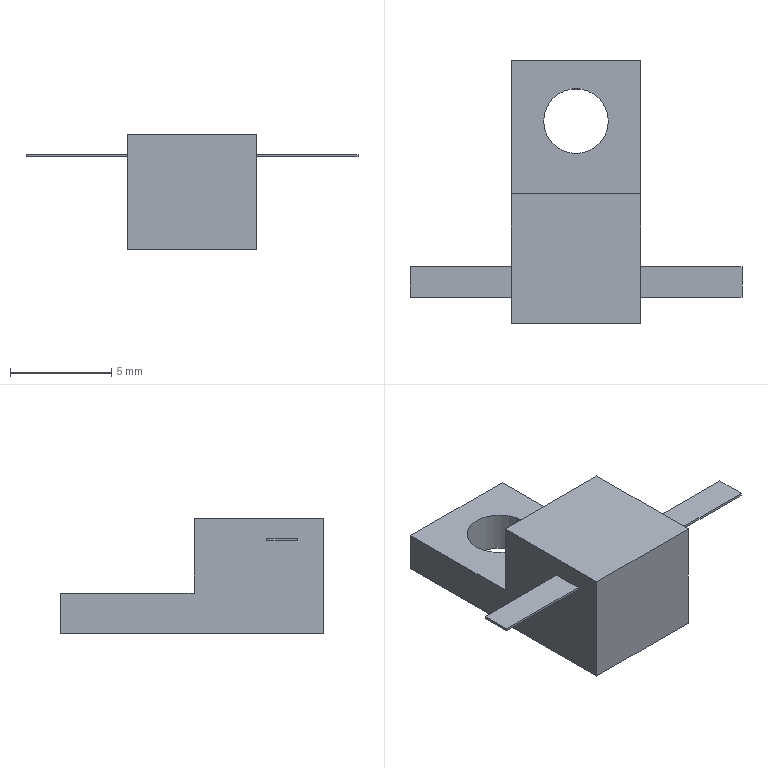Part | STEP file | RHD-50W | 1 solid | 19 faces | box 16.4 x 13 x 5.7 mm | volume 303.667 mm3 | plane 18 | cylinder 1 | commonest cylinder face diameters 3.2 x1
STEP:
#1=CARTESIAN_POINT('',(0.,0.,0.));
#2=DIRECTION('',(0.,0.,1.));
#3=DIRECTION('',(1.,0.,0.));
#4=AXIS2_PLACEMENT_3D('',#1,#2,#3);
#5=CARTESIAN_POINT('',(-120.874,-67.744,52.444));
#6=VERTEX_POINT('',#5);
#7=CARTESIAN_POINT('',(-120.874,-80.744,52.444));
#8=VERTEX_POINT('',#7);
#9=CARTESIAN_POINT('',(-120.874,-67.744,52.444));
#10=DIRECTION('',(0.,-1.,0.));
#11=VECTOR('',#10,1.);
#12=LINE('',#9,#11);
#13=CARTESIAN_POINT('',(-120.874,-67.744,54.444));
#14=DIRECTION('',(1.,0.,0.));
#15=DIRECTION('',(0.,0.,-1.));
#16=AXIS2_PLACEMENT_3D('',#13,#14,#15);
#17=PLANE('',#16);
#18=CARTESIAN_POINT('',(2.,0.));
#19=DIRECTION('',(0.,-1.));
#20=VECTOR('',#19,1.);
#21=LINE('',#18,#20);
#22=(GEOMETRIC_REPRESENTATION_CONTEXT(2)PARAMETRIC_REPRESENTATION_CONTEXT()REPRESENTATION_CONTEXT('',''));
#23=DEFINITIONAL_REPRESENTATION('',(#21),#22);
#24=PCURVE('',#17,#23);
#25=CARTESIAN_POINT('',(-117.674,-70.744,52.444));
#26=DIRECTION('',(0.,0.,1.));
#27=DIRECTION('',(1.,0.,0.));
#28=AXIS2_PLACEMENT_3D('',#25,#26,#27);
#29=PLANE('',#28);
#30=CARTESIAN_POINT('',(-3.2,3.));
#31=DIRECTION('',(0.,-1.));
#32=VECTOR('',#31,1.);
#33=LINE('',#30,#32);
#34=(GEOMETRIC_REPRESENTATION_CONTEXT(2)PARAMETRIC_REPRESENTATION_CONTEXT()REPRESENTATION_CONTEXT('',''));
#35=DEFINITIONAL_REPRESENTATION('',(#33),#34);
#36=PCURVE('',#29,#35);
#37=SURFACE_CURVE('',#12,(#24,#36),.PCURVE_S1.);
#38=EDGE_CURVE('',#6,#8,#37,.T.);
#39=ORIENTED_EDGE('',*,*,#38,.T.);
#40=CARTESIAN_POINT('',(-120.874,-80.744,58.144));
#41=VERTEX_POINT('',#40);
#42=CARTESIAN_POINT('',(-120.874,-80.744,54.444));
#43=DIRECTION('',(0.,0.,-1.));
#44=VECTOR('',#43,1.);
#45=LINE('',#42,#44);
#46=CARTESIAN_POINT('',(0.,-13.));
#47=DIRECTION('',(1.,0.));
#48=VECTOR('',#47,1.);
#49=LINE('',#46,#48);
#50=(GEOMETRIC_REPRESENTATION_CONTEXT(2)PARAMETRIC_REPRESENTATION_CONTEXT()REPRESENTATION_CONTEXT('',''));
#51=DEFINITIONAL_REPRESENTATION('',(#49),#50);
#52=PCURVE('',#17,#51);
#53=CARTESIAN_POINT('',(-120.874,-80.744,54.444));
#54=DIRECTION('',(0.,1.,0.));
#55=DIRECTION('',(0.,0.,1.));
#56=AXIS2_PLACEMENT_3D('',#53,#54,#55);
#57=PLANE('',#56);
#58=CARTESIAN_POINT('',(0.,0.));
#59=DIRECTION('',(-1.,0.));
#60=VECTOR('',#59,1.);
#61=LINE('',#58,#60);
#62=(GEOMETRIC_REPRESENTATION_CONTEXT(2)PARAMETRIC_REPRESENTATION_CONTEXT()REPRESENTATION_CONTEXT('',''));
#63=DEFINITIONAL_REPRESENTATION('',(#61),#62);
#64=PCURVE('',#57,#63);
#65=SURFACE_CURVE('',#45,(#52,#64),.PCURVE_S1.);
#66=EDGE_CURVE('',#41,#8,#65,.T.);
#67=ORIENTED_EDGE('',*,*,#66,.F.);
#68=CARTESIAN_POINT('',(-120.874,-74.344,58.144));
#69=VERTEX_POINT('',#68);
#70=CARTESIAN_POINT('',(-120.874,-74.344,58.144));
#71=DIRECTION('',(0.,-1.,0.));
#72=VECTOR('',#71,1.);
#73=LINE('',#70,#72);
#74=CARTESIAN_POINT('',(-3.7,-6.6));
#75=DIRECTION('',(0.,-1.));
#76=VECTOR('',#75,1.);
#77=LINE('',#74,#76);
#78=(GEOMETRIC_REPRESENTATION_CONTEXT(2)PARAMETRIC_REPRESENTATION_CONTEXT()REPRESENTATION_CONTEXT('',''));
#79=DEFINITIONAL_REPRESENTATION('',(#77),#78);
#80=PCURVE('',#17,#79);
#81=CARTESIAN_POINT('',(0.,0.,58.144));
#82=DIRECTION('',(0.,0.,1.));
#83=DIRECTION('',(1.,0.,0.));
#84=AXIS2_PLACEMENT_3D('',#81,#82,#83);
#85=PLANE('',#84);
#86=CARTESIAN_POINT('',(-120.874,-74.344));
#87=DIRECTION('',(0.,-1.));
#88=VECTOR('',#87,1.);
#89=LINE('',#86,#88);
#90=(GEOMETRIC_REPRESENTATION_CONTEXT(2)PARAMETRIC_REPRESENTATION_CONTEXT()REPRESENTATION_CONTEXT('',''));
#91=DEFINITIONAL_REPRESENTATION('',(#89),#90);
#92=PCURVE('',#85,#91);
#93=SURFACE_CURVE('',#73,(#80,#92),.PCURVE_S1.);
#94=EDGE_CURVE('',#69,#41,#93,.T.);
#95=ORIENTED_EDGE('',*,*,#94,.F.);
#96=CARTESIAN_POINT('',(-120.874,-74.344,54.444));
#97=VERTEX_POINT('',#96);
#98=CARTESIAN_POINT('',(-120.874,-74.344,58.144));
#99=DIRECTION('',(0.,0.,-1.));
#100=VECTOR('',#99,1.);
#101=LINE('',#98,#100);
#102=CARTESIAN_POINT('',(-3.7,-6.6));
#103=DIRECTION('',(1.,0.));
#104=VECTOR('',#103,1.);
#105=LINE('',#102,#104);
#106=(GEOMETRIC_REPRESENTATION_CONTEXT(2)PARAMETRIC_REPRESENTATION_CONTEXT()REPRESENTATION_CONTEXT('',''));
#107=DEFINITIONAL_REPRESENTATION('',(#105),#106);
#108=PCURVE('',#17,#107);
#109=CARTESIAN_POINT('',(-114.474,-74.344,58.144));
#110=DIRECTION('',(0.,-1.,0.));
#111=DIRECTION('',(0.,0.,-1.));
#112=AXIS2_PLACEMENT_3D('',#109,#110,#111);
#113=PLANE('',#112);
#114=CARTESIAN_POINT('',(0.,-6.4));
#115=DIRECTION('',(1.,0.));
#116=VECTOR('',#115,1.);
#117=LINE('',#114,#116);
#118=(GEOMETRIC_REPRESENTATION_CONTEXT(2)PARAMETRIC_REPRESENTATION_CONTEXT()REPRESENTATION_CONTEXT('',''));
#119=DEFINITIONAL_REPRESENTATION('',(#117),#118);
#120=PCURVE('',#113,#119);
#121=SURFACE_CURVE('',#101,(#108,#120),.PCURVE_S1.);
#122=EDGE_CURVE('',#69,#97,#121,.T.);
#123=ORIENTED_EDGE('',*,*,#122,.T.);
#124=CARTESIAN_POINT('',(-120.874,-67.744,54.444));
#125=VERTEX_POINT('',#124);
#126=CARTESIAN_POINT('',(-120.874,-67.744,54.444));
#127=DIRECTION('',(0.,-1.,0.));
#128=VECTOR('',#127,1.);
#129=LINE('',#126,#128);
#130=CARTESIAN_POINT('',(0.,0.));
#131=DIRECTION('',(0.,-1.));
#132=VECTOR('',#131,1.);
#133=LINE('',#130,#132);
#134=(GEOMETRIC_REPRESENTATION_CONTEXT(2)PARAMETRIC_REPRESENTATION_CONTEXT()REPRESENTATION_CONTEXT('',''));
#135=DEFINITIONAL_REPRESENTATION('',(#133),#134);
#136=PCURVE('',#17,#135);
#137=CARTESIAN_POINT('',(-117.674,-70.744,54.444));
#138=DIRECTION('',(0.,0.,1.));
#139=DIRECTION('',(1.,0.,0.));
#140=AXIS2_PLACEMENT_3D('',#137,#138,#139);
#141=PLANE('',#140);
#142=CARTESIAN_POINT('',(-3.2,3.));
#143=DIRECTION('',(0.,-1.));
#144=VECTOR('',#143,1.);
#145=LINE('',#142,#144);
#146=(GEOMETRIC_REPRESENTATION_CONTEXT(2)PARAMETRIC_REPRESENTATION_CONTEXT()REPRESENTATION_CONTEXT('',''));
#147=DEFINITIONAL_REPRESENTATION('',(#145),#146);
#148=PCURVE('',#141,#147);
#149=SURFACE_CURVE('',#129,(#136,#148),.PCURVE_S1.);
#150=EDGE_CURVE('',#125,#97,#149,.T.);
#151=ORIENTED_EDGE('',*,*,#150,.F.);
#152=CARTESIAN_POINT('',(-120.874,-67.744,54.444));
#153=DIRECTION('',(0.,0.,-1.));
#154=VECTOR('',#153,1.);
#155=LINE('',#152,#154);
#156=CARTESIAN_POINT('',(0.,0.));
#157=DIRECTION('',(1.,0.));
#158=VECTOR('',#157,1.);
#159=LINE('',#156,#158);
#160=(GEOMETRIC_REPRESENTATION_CONTEXT(2)PARAMETRIC_REPRESENTATION_CONTEXT()REPRESENTATION_CONTEXT('',''));
#161=DEFINITIONAL_REPRESENTATION('',(#159),#160);
#162=PCURVE('',#17,#161);
#163=CARTESIAN_POINT('',(-114.474,-67.744,54.444));
#164=DIRECTION('',(0.,-1.,0.));
#165=DIRECTION('',(0.,0.,-1.));
#166=AXIS2_PLACEMENT_3D('',#163,#164,#165);
#167=PLANE('',#166);
#168=CARTESIAN_POINT('',(0.,-6.4));
#169=DIRECTION('',(1.,0.));
#170=VECTOR('',#169,1.);
#171=LINE('',#168,#170);
#172=(GEOMETRIC_REPRESENTATION_CONTEXT(2)PARAMETRIC_REPRESENTATION_CONTEXT()REPRESENTATION_CONTEXT('',''));
#173=DEFINITIONAL_REPRESENTATION('',(#171),#172);
#174=PCURVE('',#167,#173);
#175=SURFACE_CURVE('',#155,(#162,#174),.PCURVE_S1.);
#176=EDGE_CURVE('',#125,#6,#175,.T.);
#177=ORIENTED_EDGE('',*,*,#176,.T.);
#178=EDGE_LOOP('',(#39,#67,#95,#123,#151,#177));
#179=FACE_BOUND('',#178,.T.);
#180=CARTESIAN_POINT('',(-120.874,-79.444,57.024));
#181=VERTEX_POINT('',#180);
#182=CARTESIAN_POINT('',(-120.874,-79.444,57.144));
#183=VERTEX_POINT('',#182);
#184=CARTESIAN_POINT('',(-120.874,-79.444,57.024));
#185=DIRECTION('',(0.,0.,1.));
#186=VECTOR('',#185,1.);
#187=LINE('',#184,#186);
#188=CARTESIAN_POINT('',(-2.58,-11.7));
#189=DIRECTION('',(-1.,0.));
#190=VECTOR('',#189,1.);
#191=LINE('',#188,#190);
#192=(GEOMETRIC_REPRESENTATION_CONTEXT(2)PARAMETRIC_REPRESENTATION_CONTEXT()REPRESENTATION_CONTEXT('',''));
#193=DEFINITIONAL_REPRESENTATION('',(#191),#192);
#194=PCURVE('',#17,#193);
#195=CARTESIAN_POINT('',(-125.874,-79.444,57.024));
#196=DIRECTION('',(0.,1.,0.));
#197=DIRECTION('',(0.,0.,1.));
#198=AXIS2_PLACEMENT_3D('',#195,#196,#197);
#199=PLANE('',#198);
#200=CARTESIAN_POINT('',(0.,5.));
#201=DIRECTION('',(1.,0.));
#202=VECTOR('',#201,1.);
#203=LINE('',#200,#202);
#204=(GEOMETRIC_REPRESENTATION_CONTEXT(2)PARAMETRIC_REPRESENTATION_CONTEXT()REPRESENTATION_CONTEXT('',''));
#205=DEFINITIONAL_REPRESENTATION('',(#203),#204);
#206=PCURVE('',#199,#205);
#207=SURFACE_CURVE('',#187,(#194,#206),.PCURVE_S1.);
#208=EDGE_CURVE('',#181,#183,#207,.T.);
#209=ORIENTED_EDGE('',*,*,#208,.F.);
#210=CARTESIAN_POINT('',(-120.874,-77.944,57.024));
#211=VERTEX_POINT('',#210);
#212=CARTESIAN_POINT('',(-120.874,-77.944,57.024));
#213=DIRECTION('',(0.,-1.,0.));
#214=VECTOR('',#213,1.);
#215=LINE('',#212,#214);
#216=CARTESIAN_POINT('',(-2.58,-10.2));
#217=DIRECTION('',(0.,-1.));
#218=VECTOR('',#217,1.);
#219=LINE('',#216,#218);
#220=(GEOMETRIC_REPRESENTATION_CONTEXT(2)PARAMETRIC_REPRESENTATION_CONTEXT()REPRESENTATION_CONTEXT('',''));
#221=DEFINITIONAL_REPRESENTATION('',(#219),#220);
#222=PCURVE('',#17,#221);
#223=CARTESIAN_POINT('',(-125.874,-77.944,57.024));
#224=DIRECTION('',(0.,0.,1.));
#225=DIRECTION('',(1.,0.,0.));
#226=AXIS2_PLACEMENT_3D('',#223,#224,#225);
#227=PLANE('',#226);
#228=CARTESIAN_POINT('',(5.,0.));
#229=DIRECTION('',(0.,-1.));
#230=VECTOR('',#229,1.);
#231=LINE('',#228,#230);
#232=(GEOMETRIC_REPRESENTATION_CONTEXT(2)PARAMETRIC_REPRESENTATION_CONTEXT()REPRESENTATION_CONTEXT('',''));
#233=DEFINITIONAL_REPRESENTATION('',(#231),#232);
#234=PCURVE('',#227,#233);
#235=SURFACE_CURVE('',#215,(#222,#234),.PCURVE_S1.);
#236=EDGE_CURVE('',#211,#181,#235,.T.);
#237=ORIENTED_EDGE('',*,*,#236,.F.);
#238=CARTESIAN_POINT('',(-120.874,-77.944,57.144));
#239=VERTEX_POINT('',#238);
#240=CARTESIAN_POINT('',(-120.874,-77.944,57.144));
#241=DIRECTION('',(0.,0.,-1.));
#242=VECTOR('',#241,1.);
#243=LINE('',#240,#242);
#244=CARTESIAN_POINT('',(-2.7,-10.2));
#245=DIRECTION('',(1.,0.));
#246=VECTOR('',#245,1.);
#247=LINE('',#244,#246);
#248=(GEOMETRIC_REPRESENTATION_CONTEXT(2)PARAMETRIC_REPRESENTATION_CONTEXT()REPRESENTATION_CONTEXT('',''));
#249=DEFINITIONAL_REPRESENTATION('',(#247),#248);
#250=PCURVE('',#17,#249);
#251=CARTESIAN_POINT('',(-125.874,-77.944,57.144));
#252=DIRECTION('',(0.,-1.,0.));
#253=DIRECTION('',(0.,0.,-1.));
#254=AXIS2_PLACEMENT_3D('',#251,#252,#253);
#255=PLANE('',#254);
#256=CARTESIAN_POINT('',(0.,5.));
#257=DIRECTION('',(1.,0.));
#258=VECTOR('',#257,1.);
#259=LINE('',#256,#258);
#260=(GEOMETRIC_REPRESENTATION_CONTEXT(2)PARAMETRIC_REPRESENTATION_CONTEXT()REPRESENTATION_CONTEXT('',''));
#261=DEFINITIONAL_REPRESENTATION('',(#259),#260);
#262=PCURVE('',#255,#261);
#263=SURFACE_CURVE('',#243,(#250,#262),.PCURVE_S1.);
#264=EDGE_CURVE('',#239,#211,#263,.T.);
#265=ORIENTED_EDGE('',*,*,#264,.F.);
#266=CARTESIAN_POINT('',(-120.874,-79.444,57.144));
#267=DIRECTION('',(0.,1.,0.));
#268=VECTOR('',#267,1.);
#269=LINE('',#266,#268);
#270=CARTESIAN_POINT('',(-2.7,-11.7));
#271=DIRECTION('',(0.,1.));
#272=VECTOR('',#271,1.);
#273=LINE('',#270,#272);
#274=(GEOMETRIC_REPRESENTATION_CONTEXT(2)PARAMETRIC_REPRESENTATION_CONTEXT()REPRESENTATION_CONTEXT('',''));
#275=DEFINITIONAL_REPRESENTATION('',(#273),#274);
#276=PCURVE('',#17,#275);
#277=CARTESIAN_POINT('',(-125.874,-79.444,57.144));
#278=DIRECTION('',(0.,0.,-1.));
#279=DIRECTION('',(-1.,0.,0.));
#280=AXIS2_PLACEMENT_3D('',#277,#278,#279);
#281=PLANE('',#280);
#282=CARTESIAN_POINT('',(-5.,0.));
#283=DIRECTION('',(0.,1.));
#284=VECTOR('',#283,1.);
#285=LINE('',#282,#284);
#286=(GEOMETRIC_REPRESENTATION_CONTEXT(2)PARAMETRIC_REPRESENTATION_CONTEXT()REPRESENTATION_CONTEXT('',''));
#287=DEFINITIONAL_REPRESENTATION('',(#285),#286);
#288=PCURVE('',#281,#287);
#289=SURFACE_CURVE('',#269,(#276,#288),.PCURVE_S1.);
#290=EDGE_CURVE('',#183,#239,#289,.T.);
#291=ORIENTED_EDGE('',*,*,#290,.F.);
#292=EDGE_LOOP('',(#209,#237,#265,#291));
#293=FACE_BOUND('',#292,.T.);
#294=ADVANCED_FACE('',(#179,#293),#17,.F.);
#295=CARTESIAN_POINT('',(-114.474,-80.744,52.444));
#296=VERTEX_POINT('',#295);
#297=CARTESIAN_POINT('',(-114.474,-67.744,52.444));
#298=VERTEX_POINT('',#297);
#299=CARTESIAN_POINT('',(-114.474,-80.744,52.444));
#300=DIRECTION('',(0.,1.,0.));
#301=VECTOR('',#300,1.);
#302=LINE('',#299,#301);
#303=CARTESIAN_POINT('',(-114.474,-80.744,54.444));
#304=DIRECTION('',(-1.,0.,0.));
#305=DIRECTION('',(0.,0.,1.));
#306=AXIS2_PLACEMENT_3D('',#303,#304,#305);
#307=PLANE('',#306);
#308=CARTESIAN_POINT('',(-2.,0.));
#309=DIRECTION('',(0.,1.));
#310=VECTOR('',#309,1.);
#311=LINE('',#308,#310);
#312=(GEOMETRIC_REPRESENTATION_CONTEXT(2)PARAMETRIC_REPRESENTATION_CONTEXT()REPRESENTATION_CONTEXT('',''));
#313=DEFINITIONAL_REPRESENTATION('',(#311),#312);
#314=PCURVE('',#307,#313);
#315=CARTESIAN_POINT('',(3.2,-10.));
#316=DIRECTION('',(0.,1.));
#317=VECTOR('',#316,1.);
#318=LINE('',#315,#317);
#319=(GEOMETRIC_REPRESENTATION_CONTEXT(2)PARAMETRIC_REPRESENTATION_CONTEXT()REPRESENTATION_CONTEXT('',''));
#320=DEFINITIONAL_REPRESENTATION('',(#318),#319);
#321=PCURVE('',#29,#320);
#322=SURFACE_CURVE('',#302,(#314,#321),.PCURVE_S1.);
#323=EDGE_CURVE('',#296,#298,#322,.T.);
#324=ORIENTED_EDGE('',*,*,#323,.T.);
#325=CARTESIAN_POINT('',(-114.474,-67.744,54.444));
#326=VERTEX_POINT('',#325);
#327=CARTESIAN_POINT('',(-114.474,-67.744,54.444));
#328=DIRECTION('',(0.,0.,-1.));
#329=VECTOR('',#328,1.);
#330=LINE('',#327,#329);
#331=CARTESIAN_POINT('',(0.,13.));
#332=DIRECTION('',(-1.,0.));
#333=VECTOR('',#332,1.);
#334=LINE('',#331,#333);
#335=(GEOMETRIC_REPRESENTATION_CONTEXT(2)PARAMETRIC_REPRESENTATION_CONTEXT()REPRESENTATION_CONTEXT('',''));
#336=DEFINITIONAL_REPRESENTATION('',(#334),#335);
#337=PCURVE('',#307,#336);
#338=CARTESIAN_POINT('',(0.,0.));
#339=DIRECTION('',(1.,0.));
#340=VECTOR('',#339,1.);
#341=LINE('',#338,#340);
#342=(GEOMETRIC_REPRESENTATION_CONTEXT(2)PARAMETRIC_REPRESENTATION_CONTEXT()REPRESENTATION_CONTEXT('',''));
#343=DEFINITIONAL_REPRESENTATION('',(#341),#342);
#344=PCURVE('',#167,#343);
#345=SURFACE_CURVE('',#330,(#337,#344),.PCURVE_S1.);
#346=EDGE_CURVE('',#326,#298,#345,.T.);
#347=ORIENTED_EDGE('',*,*,#346,.F.);
#348=CARTESIAN_POINT('',(-114.474,-74.344,54.444));
#349=VERTEX_POINT('',#348);
#350=CARTESIAN_POINT('',(-114.474,-80.744,54.444));
#351=DIRECTION('',(0.,1.,0.));
#352=VECTOR('',#351,1.);
#353=LINE('',#350,#352);
#354=CARTESIAN_POINT('',(0.,0.));
#355=DIRECTION('',(0.,1.));
#356=VECTOR('',#355,1.);
#357=LINE('',#354,#356);
#358=(GEOMETRIC_REPRESENTATION_CONTEXT(2)PARAMETRIC_REPRESENTATION_CONTEXT()REPRESENTATION_CONTEXT('',''));
#359=DEFINITIONAL_REPRESENTATION('',(#357),#358);
#360=PCURVE('',#307,#359);
#361=CARTESIAN_POINT('',(3.2,-10.));
#362=DIRECTION('',(0.,1.));
#363=VECTOR('',#362,1.);
#364=LINE('',#361,#363);
#365=(GEOMETRIC_REPRESENTATION_CONTEXT(2)PARAMETRIC_REPRESENTATION_CONTEXT()REPRESENTATION_CONTEXT('',''));
#366=DEFINITIONAL_REPRESENTATION('',(#364),#365);
#367=PCURVE('',#141,#366);
#368=SURFACE_CURVE('',#353,(#360,#367),.PCURVE_S1.);
#369=EDGE_CURVE('',#349,#326,#368,.T.);
#370=ORIENTED_EDGE('',*,*,#369,.F.);
#371=CARTESIAN_POINT('',(-114.474,-74.344,58.144));
#372=VERTEX_POINT('',#371);
#373=CARTESIAN_POINT('',(-114.474,-74.344,58.144));
#374=DIRECTION('',(0.,0.,-1.));
#375=VECTOR('',#374,1.);
#376=LINE('',#373,#375);
#377=CARTESIAN_POINT('',(3.7,6.4));
#378=DIRECTION('',(-1.,0.));
#379=VECTOR('',#378,1.);
#380=LINE('',#377,#379);
#381=(GEOMETRIC_REPRESENTATION_CONTEXT(2)PARAMETRIC_REPRESENTATION_CONTEXT()REPRESENTATION_CONTEXT('',''));
#382=DEFINITIONAL_REPRESENTATION('',(#380),#381);
#383=PCURVE('',#307,#382);
#384=CARTESIAN_POINT('',(0.,0.));
#385=DIRECTION('',(1.,0.));
#386=VECTOR('',#385,1.);
#387=LINE('',#384,#386);
#388=(GEOMETRIC_REPRESENTATION_CONTEXT(2)PARAMETRIC_REPRESENTATION_CONTEXT()REPRESENTATION_CONTEXT('',''));
#389=DEFINITIONAL_REPRESENTATION('',(#387),#388);
#390=PCURVE('',#113,#389);
#391=SURFACE_CURVE('',#376,(#383,#390),.PCURVE_S1.);
#392=EDGE_CURVE('',#372,#349,#391,.T.);
#393=ORIENTED_EDGE('',*,*,#392,.F.);
#394=CARTESIAN_POINT('',(-114.474,-80.744,58.144));
#395=VERTEX_POINT('',#394);
#396=CARTESIAN_POINT('',(-114.474,-80.744,58.144));
#397=DIRECTION('',(0.,1.,0.));
#398=VECTOR('',#397,1.);
#399=LINE('',#396,#398);
#400=CARTESIAN_POINT('',(3.7,0.));
#401=DIRECTION('',(0.,1.));
#402=VECTOR('',#401,1.);
#403=LINE('',#400,#402);
#404=(GEOMETRIC_REPRESENTATION_CONTEXT(2)PARAMETRIC_REPRESENTATION_CONTEXT()REPRESENTATION_CONTEXT('',''));
#405=DEFINITIONAL_REPRESENTATION('',(#403),#404);
#406=PCURVE('',#307,#405);
#407=CARTESIAN_POINT('',(-114.474,-80.744));
#408=DIRECTION('',(0.,1.));
#409=VECTOR('',#408,1.);
#410=LINE('',#407,#409);
#411=(GEOMETRIC_REPRESENTATION_CONTEXT(2)PARAMETRIC_REPRESENTATION_CONTEXT()REPRESENTATION_CONTEXT('',''));
#412=DEFINITIONAL_REPRESENTATION('',(#410),#411);
#413=PCURVE('',#85,#412);
#414=SURFACE_CURVE('',#399,(#406,#413),.PCURVE_S1.);
#415=EDGE_CURVE('',#395,#372,#414,.T.);
#416=ORIENTED_EDGE('',*,*,#415,.F.);
#417=CARTESIAN_POINT('',(-114.474,-80.744,54.444));
#418=DIRECTION('',(0.,0.,-1.));
#419=VECTOR('',#418,1.);
#420=LINE('',#417,#419);
#421=CARTESIAN_POINT('',(0.,0.));
#422=DIRECTION('',(-1.,0.));
#423=VECTOR('',#422,1.);
#424=LINE('',#421,#423);
#425=(GEOMETRIC_REPRESENTATION_CONTEXT(2)PARAMETRIC_REPRESENTATION_CONTEXT()REPRESENTATION_CONTEXT('',''));
#426=DEFINITIONAL_REPRESENTATION('',(#424),#425);
#427=PCURVE('',#307,#426);
#428=CARTESIAN_POINT('',(0.,6.4));
#429=DIRECTION('',(-1.,0.));
#430=VECTOR('',#429,1.);
#431=LINE('',#428,#430);
#432=(GEOMETRIC_REPRESENTATION_CONTEXT(2)PARAMETRIC_REPRESENTATION_CONTEXT()REPRESENTATION_CONTEXT('',''));
#433=DEFINITIONAL_REPRESENTATION('',(#431),#432);
#434=PCURVE('',#57,#433);
#435=SURFACE_CURVE('',#420,(#427,#434),.PCURVE_S1.);
#436=EDGE_CURVE('',#395,#296,#435,.T.);
#437=ORIENTED_EDGE('',*,*,#436,.T.);
#438=EDGE_LOOP('',(#324,#347,#370,#393,#416,#437));
#439=FACE_BOUND('',#438,.T.);
#440=CARTESIAN_POINT('',(-114.474,-79.444,57.144));
#441=VERTEX_POINT('',#440);
#442=CARTESIAN_POINT('',(-114.474,-79.444,57.024));
#443=VERTEX_POINT('',#442);
#444=CARTESIAN_POINT('',(-114.474,-79.444,57.144));
#445=DIRECTION('',(0.,0.,-1.));
#446=VECTOR('',#445,1.);
#447=LINE('',#444,#446);
#448=CARTESIAN_POINT('',(2.7,1.3));
#449=DIRECTION('',(-1.,0.));
#450=VECTOR('',#449,1.);
#451=LINE('',#448,#450);
#452=(GEOMETRIC_REPRESENTATION_CONTEXT(2)PARAMETRIC_REPRESENTATION_CONTEXT()REPRESENTATION_CONTEXT('',''));
#453=DEFINITIONAL_REPRESENTATION('',(#451),#452);
#454=PCURVE('',#307,#453);
#455=CARTESIAN_POINT('',(-109.474,-79.444,57.144));
#456=DIRECTION('',(0.,1.,0.));
#457=DIRECTION('',(0.,0.,1.));
#458=AXIS2_PLACEMENT_3D('',#455,#456,#457);
#459=PLANE('',#458);
#460=CARTESIAN_POINT('',(0.,-5.));
#461=DIRECTION('',(-1.,0.));
#462=VECTOR('',#461,1.);
#463=LINE('',#460,#462);
#464=(GEOMETRIC_REPRESENTATION_CONTEXT(2)PARAMETRIC_REPRESENTATION_CONTEXT()REPRESENTATION_CONTEXT('',''));
#465=DEFINITIONAL_REPRESENTATION('',(#463),#464);
#466=PCURVE('',#459,#465);
#467=SURFACE_CURVE('',#447,(#454,#466),.PCURVE_S1.);
#468=EDGE_CURVE('',#441,#443,#467,.T.);
#469=ORIENTED_EDGE('',*,*,#468,.F.);
#470=CARTESIAN_POINT('',(-114.474,-77.944,57.144));
#471=VERTEX_POINT('',#470);
#472=CARTESIAN_POINT('',(-114.474,-77.944,57.144));
#473=DIRECTION('',(0.,-1.,0.));
#474=VECTOR('',#473,1.);
#475=LINE('',#472,#474);
#476=CARTESIAN_POINT('',(2.7,2.8));
#477=DIRECTION('',(0.,-1.));
#478=VECTOR('',#477,1.);
#479=LINE('',#476,#478);
#480=(GEOMETRIC_REPRESENTATION_CONTEXT(2)PARAMETRIC_REPRESENTATION_CONTEXT()REPRESENTATION_CONTEXT('',''));
#481=DEFINITIONAL_REPRESENTATION('',(#479),#480);
#482=PCURVE('',#307,#481);
#483=CARTESIAN_POINT('',(-109.474,-77.944,57.144));
#484=DIRECTION('',(0.,0.,-1.));
#485=DIRECTION('',(-1.,0.,0.));
#486=AXIS2_PLACEMENT_3D('',#483,#484,#485);
#487=PLANE('',#486);
#488=CARTESIAN_POINT('',(5.,0.));
#489=DIRECTION('',(0.,-1.));
#490=VECTOR('',#489,1.);
#491=LINE('',#488,#490);
#492=(GEOMETRIC_REPRESENTATION_CONTEXT(2)PARAMETRIC_REPRESENTATION_CONTEXT()REPRESENTATION_CONTEXT('',''));
#493=DEFINITIONAL_REPRESENTATION('',(#491),#492);
#494=PCURVE('',#487,#493);
#495=SURFACE_CURVE('',#475,(#482,#494),.PCURVE_S1.);
#496=EDGE_CURVE('',#471,#441,#495,.T.);
#497=ORIENTED_EDGE('',*,*,#496,.F.);
#498=CARTESIAN_POINT('',(-114.474,-77.944,57.024));
#499=VERTEX_POINT('',#498);
#500=CARTESIAN_POINT('',(-114.474,-77.944,57.024));
#501=DIRECTION('',(0.,0.,1.));
#502=VECTOR('',#501,1.);
#503=LINE('',#500,#502);
#504=CARTESIAN_POINT('',(2.58,2.8));
#505=DIRECTION('',(1.,0.));
#506=VECTOR('',#505,1.);
#507=LINE('',#504,#506);
#508=(GEOMETRIC_REPRESENTATION_CONTEXT(2)PARAMETRIC_REPRESENTATION_CONTEXT()REPRESENTATION_CONTEXT('',''));
#509=DEFINITIONAL_REPRESENTATION('',(#507),#508);
#510=PCURVE('',#307,#509);
#511=CARTESIAN_POINT('',(-109.474,-77.944,57.024));
#512=DIRECTION('',(0.,-1.,0.));
#513=DIRECTION('',(0.,0.,-1.));
#514=AXIS2_PLACEMENT_3D('',#511,#512,#513);
#515=PLANE('',#514);
#516=CARTESIAN_POINT('',(0.,-5.));
#517=DIRECTION('',(-1.,0.));
#518=VECTOR('',#517,1.);
#519=LINE('',#516,#518);
#520=(GEOMETRIC_REPRESENTATION_CONTEXT(2)PARAMETRIC_REPRESENTATION_CONTEXT()REPRESENTATION_CONTEXT('',''));
#521=DEFINITIONAL_REPRESENTATION('',(#519),#520);
#522=PCURVE('',#515,#521);
#523=SURFACE_CURVE('',#503,(#510,#522),.PCURVE_S1.);
#524=EDGE_CURVE('',#499,#471,#523,.T.);
#525=ORIENTED_EDGE('',*,*,#524,.F.);
#526=CARTESIAN_POINT('',(-114.474,-79.444,57.024));
#527=DIRECTION('',(0.,1.,0.));
#528=VECTOR('',#527,1.);
#529=LINE('',#526,#528);
#530=CARTESIAN_POINT('',(2.58,1.3));
#531=DIRECTION('',(0.,1.));
#532=VECTOR('',#531,1.);
#533=LINE('',#530,#532);
#534=(GEOMETRIC_REPRESENTATION_CONTEXT(2)PARAMETRIC_REPRESENTATION_CONTEXT()REPRESENTATION_CONTEXT('',''));
#535=DEFINITIONAL_REPRESENTATION('',(#533),#534);
#536=PCURVE('',#307,#535);
#537=CARTESIAN_POINT('',(-109.474,-79.444,57.024));
#538=DIRECTION('',(0.,0.,1.));
#539=DIRECTION('',(1.,0.,0.));
#540=AXIS2_PLACEMENT_3D('',#537,#538,#539);
#541=PLANE('',#540);
#542=CARTESIAN_POINT('',(-5.,0.));
#543=DIRECTION('',(0.,1.));
#544=VECTOR('',#543,1.);
#545=LINE('',#542,#544);
#546=(GEOMETRIC_REPRESENTATION_CONTEXT(2)PARAMETRIC_REPRESENTATION_CONTEXT()REPRESENTATION_CONTEXT('',''));
#547=DEFINITIONAL_REPRESENTATION('',(#545),#546);
#548=PCURVE('',#541,#547);
#549=SURFACE_CURVE('',#529,(#536,#548),.PCURVE_S1.);
#550=EDGE_CURVE('',#443,#499,#549,.T.);
#551=ORIENTED_EDGE('',*,*,#550,.F.);
#552=EDGE_LOOP('',(#469,#497,#525,#551));
#553=FACE_BOUND('',#552,.T.);
#554=ADVANCED_FACE('',(#439,#553),#307,.F.);
#555=CARTESIAN_POINT('',(-120.874,-80.744,52.444));
#556=DIRECTION('',(1.,0.,0.));
#557=VECTOR('',#556,1.);
#558=LINE('',#555,#557);
#559=CARTESIAN_POINT('',(-2.,0.));
#560=DIRECTION('',(0.,1.));
#561=VECTOR('',#560,1.);
#562=LINE('',#559,#561);
#563=(GEOMETRIC_REPRESENTATION_CONTEXT(2)PARAMETRIC_REPRESENTATION_CONTEXT()REPRESENTATION_CONTEXT('',''));
#564=DEFINITIONAL_REPRESENTATION('',(#562),#563);
#565=PCURVE('',#57,#564);
#566=CARTESIAN_POINT('',(-3.2,-10.));
#567=DIRECTION('',(1.,0.));
#568=VECTOR('',#567,1.);
#569=LINE('',#566,#568);
#570=(GEOMETRIC_REPRESENTATION_CONTEXT(2)PARAMETRIC_REPRESENTATION_CONTEXT()REPRESENTATION_CONTEXT('',''));
#571=DEFINITIONAL_REPRESENTATION('',(#569),#570);
#572=PCURVE('',#29,#571);
#573=SURFACE_CURVE('',#558,(#565,#572),.PCURVE_S1.);
#574=EDGE_CURVE('',#8,#296,#573,.T.);
#575=ORIENTED_EDGE('',*,*,#574,.T.);
#576=ORIENTED_EDGE('',*,*,#436,.F.);
#577=CARTESIAN_POINT('',(-120.874,-80.744,58.144));
#578=DIRECTION('',(1.,0.,0.));
#579=VECTOR('',#578,1.);
#580=LINE('',#577,#579);
#581=CARTESIAN_POINT('',(3.7,0.));
#582=DIRECTION('',(0.,1.));
#583=VECTOR('',#582,1.);
#584=LINE('',#581,#583);
#585=(GEOMETRIC_REPRESENTATION_CONTEXT(2)PARAMETRIC_REPRESENTATION_CONTEXT()REPRESENTATION_CONTEXT('',''));
#586=DEFINITIONAL_REPRESENTATION('',(#584),#585);
#587=PCURVE('',#57,#586);
#588=CARTESIAN_POINT('',(-120.874,-80.744));
#589=DIRECTION('',(1.,0.));
#590=VECTOR('',#589,1.);
#591=LINE('',#588,#590);
#592=(GEOMETRIC_REPRESENTATION_CONTEXT(2)PARAMETRIC_REPRESENTATION_CONTEXT()REPRESENTATION_CONTEXT('',''));
#593=DEFINITIONAL_REPRESENTATION('',(#591),#592);
#594=PCURVE('',#85,#593);
#595=SURFACE_CURVE('',#580,(#587,#594),.PCURVE_S1.);
#596=EDGE_CURVE('',#41,#395,#595,.T.);
#597=ORIENTED_EDGE('',*,*,#596,.F.);
#598=ORIENTED_EDGE('',*,*,#66,.T.);
#599=EDGE_LOOP('',(#575,#576,#597,#598));
#600=FACE_BOUND('',#599,.T.);
#601=ADVANCED_FACE('',(#600),#57,.F.);
#602=CARTESIAN_POINT('',(-114.474,-67.744,52.444));
#603=DIRECTION('',(-1.,0.,0.));
#604=VECTOR('',#603,1.);
#605=LINE('',#602,#604);
#606=CARTESIAN_POINT('',(2.,0.));
#607=DIRECTION('',(0.,-1.));
#608=VECTOR('',#607,1.);
#609=LINE('',#606,#608);
#610=(GEOMETRIC_REPRESENTATION_CONTEXT(2)PARAMETRIC_REPRESENTATION_CONTEXT()REPRESENTATION_CONTEXT('',''));
#611=DEFINITIONAL_REPRESENTATION('',(#609),#610);
#612=PCURVE('',#167,#611);
#613=CARTESIAN_POINT('',(3.2,3.));
#614=DIRECTION('',(-1.,0.));
#615=VECTOR('',#614,1.);
#616=LINE('',#613,#615);
#617=(GEOMETRIC_REPRESENTATION_CONTEXT(2)PARAMETRIC_REPRESENTATION_CONTEXT()REPRESENTATION_CONTEXT('',''));
#618=DEFINITIONAL_REPRESENTATION('',(#616),#617);
#619=PCURVE('',#29,#618);
#620=SURFACE_CURVE('',#605,(#612,#619),.PCURVE_S1.);
#621=EDGE_CURVE('',#298,#6,#620,.T.);
#622=ORIENTED_EDGE('',*,*,#621,.T.);
#623=ORIENTED_EDGE('',*,*,#176,.F.);
#624=CARTESIAN_POINT('',(-114.474,-67.744,54.444));
#625=DIRECTION('',(-1.,0.,0.));
#626=VECTOR('',#625,1.);
#627=LINE('',#624,#626);
#628=CARTESIAN_POINT('',(0.,0.));
#629=DIRECTION('',(0.,-1.));
#630=VECTOR('',#629,1.);
#631=LINE('',#628,#630);
#632=(GEOMETRIC_REPRESENTATION_CONTEXT(2)PARAMETRIC_REPRESENTATION_CONTEXT()REPRESENTATION_CONTEXT('',''));
#633=DEFINITIONAL_REPRESENTATION('',(#631),#632);
#634=PCURVE('',#167,#633);
#635=CARTESIAN_POINT('',(3.2,3.));
#636=DIRECTION('',(-1.,0.));
#637=VECTOR('',#636,1.);
#638=LINE('',#635,#637);
#639=(GEOMETRIC_REPRESENTATION_CONTEXT(2)PARAMETRIC_REPRESENTATION_CONTEXT()REPRESENTATION_CONTEXT('',''));
#640=DEFINITIONAL_REPRESENTATION('',(#638),#639);
#641=PCURVE('',#141,#640);
#642=SURFACE_CURVE('',#627,(#634,#641),.PCURVE_S1.);
#643=EDGE_CURVE('',#326,#125,#642,.T.);
#644=ORIENTED_EDGE('',*,*,#643,.F.);
#645=ORIENTED_EDGE('',*,*,#346,.T.);
#646=EDGE_LOOP('',(#622,#623,#644,#645));
#647=FACE_BOUND('',#646,.T.);
#648=ADVANCED_FACE('',(#647),#167,.F.);
#649=CARTESIAN_POINT('',(-119.274,-70.744,54.444));
#650=VERTEX_POINT('',#649);
#651=CARTESIAN_POINT('',(-117.674,-70.744,54.444));
#652=DIRECTION('',(0.,0.,1.));
#653=DIRECTION('',(-1.,0.,0.));
#654=AXIS2_PLACEMENT_3D('',#651,#652,#653);
#655=CIRCLE('',#654,1.6);
#656=CARTESIAN_POINT('',(-117.674,-70.744,54.444));
#657=DIRECTION('',(0.,0.,-1.));
#658=DIRECTION('',(-1.,0.,0.));
#659=AXIS2_PLACEMENT_3D('',#656,#657,#658);
#660=CYLINDRICAL_SURFACE('',#659,1.6);
#661=CARTESIAN_POINT('',(6.283,0.));
#662=DIRECTION('',(-1.,0.));
#663=VECTOR('',#662,1.);
#664=LINE('',#661,#663);
#665=(GEOMETRIC_REPRESENTATION_CONTEXT(2)PARAMETRIC_REPRESENTATION_CONTEXT()REPRESENTATION_CONTEXT('',''));
#666=DEFINITIONAL_REPRESENTATION('',(#664),#665);
#667=PCURVE('',#660,#666);
#668=CARTESIAN_POINT('',(0.,0.));
#669=DIRECTION('',(-1.,0.));
#670=AXIS2_PLACEMENT_2D('',#668,#669);
#671=CIRCLE('',#670,1.6);
#672=(GEOMETRIC_REPRESENTATION_CONTEXT(2)PARAMETRIC_REPRESENTATION_CONTEXT()REPRESENTATION_CONTEXT('',''));
#673=DEFINITIONAL_REPRESENTATION('',(#671),#672);
#674=PCURVE('',#141,#673);
#675=SURFACE_CURVE('',#655,(#667,#674),.PCURVE_S1.);
#676=EDGE_CURVE('',#650,#650,#675,.T.);
#677=ORIENTED_EDGE('',*,*,#676,.F.);
#678=CARTESIAN_POINT('',(-119.274,-70.744,52.444));
#679=VERTEX_POINT('',#678);
#680=CARTESIAN_POINT('',(-119.274,-70.744,54.444));
#681=CARTESIAN_POINT('',(-119.274,-70.744,52.444));
#682=B_SPLINE_CURVE_WITH_KNOTS('',1,(#680,#681),.UNSPECIFIED.,.F.,.F.,(2,2),(0.,2.),.PIECEWISE_BEZIER_KNOTS.);
#683=CARTESIAN_POINT('',(6.283,0.));
#684=DIRECTION('',(0.,1.));
#685=VECTOR('',#684,1.);
#686=LINE('',#683,#685);
#687=(GEOMETRIC_REPRESENTATION_CONTEXT(2)PARAMETRIC_REPRESENTATION_CONTEXT()REPRESENTATION_CONTEXT('',''));
#688=DEFINITIONAL_REPRESENTATION('',(#686),#687);
#689=PCURVE('',#660,#688);
#690=CARTESIAN_POINT('',(0.,0.));
#691=DIRECTION('',(0.,1.));
#692=VECTOR('',#691,1.);
#693=LINE('',#690,#692);
#694=(GEOMETRIC_REPRESENTATION_CONTEXT(2)PARAMETRIC_REPRESENTATION_CONTEXT()REPRESENTATION_CONTEXT('',''));
#695=DEFINITIONAL_REPRESENTATION('',(#693),#694);
#696=PCURVE('',#660,#695);
#697=SEAM_CURVE('',#682,(#689,#696),.PCURVE_S1.);
#698=EDGE_CURVE('',#650,#679,#697,.T.);
#699=ORIENTED_EDGE('',*,*,#698,.T.);
#700=CARTESIAN_POINT('',(-117.674,-70.744,52.444));
#701=DIRECTION('',(0.,0.,1.));
#702=DIRECTION('',(-1.,0.,0.));
#703=AXIS2_PLACEMENT_3D('',#700,#701,#702);
#704=CIRCLE('',#703,1.6);
#705=CARTESIAN_POINT('',(6.283,2.));
#706=DIRECTION('',(-1.,0.));
#707=VECTOR('',#706,1.);
#708=LINE('',#705,#707);
#709=(GEOMETRIC_REPRESENTATION_CONTEXT(2)PARAMETRIC_REPRESENTATION_CONTEXT()REPRESENTATION_CONTEXT('',''));
#710=DEFINITIONAL_REPRESENTATION('',(#708),#709);
#711=PCURVE('',#660,#710);
#712=CARTESIAN_POINT('',(0.,0.));
#713=DIRECTION('',(-1.,0.));
#714=AXIS2_PLACEMENT_2D('',#712,#713);
#715=CIRCLE('',#714,1.6);
#716=(GEOMETRIC_REPRESENTATION_CONTEXT(2)PARAMETRIC_REPRESENTATION_CONTEXT()REPRESENTATION_CONTEXT('',''));
#717=DEFINITIONAL_REPRESENTATION('',(#715),#716);
#718=PCURVE('',#29,#717);
#719=SURFACE_CURVE('',#704,(#711,#718),.PCURVE_S1.);
#720=EDGE_CURVE('',#679,#679,#719,.T.);
#721=ORIENTED_EDGE('',*,*,#720,.T.);
#722=ORIENTED_EDGE('',*,*,#698,.F.);
#723=EDGE_LOOP('',(#677,#699,#721,#722));
#724=FACE_BOUND('',#723,.F.);
#725=ADVANCED_FACE('',(#724),#660,.F.);
#726=CARTESIAN_POINT('',(-114.474,-74.344,54.444));
#727=DIRECTION('',(-1.,0.,0.));
#728=VECTOR('',#727,1.);
#729=LINE('',#726,#728);
#730=CARTESIAN_POINT('',(3.2,-3.6));
#731=DIRECTION('',(-1.,0.));
#732=VECTOR('',#731,1.);
#733=LINE('',#730,#732);
#734=(GEOMETRIC_REPRESENTATION_CONTEXT(2)PARAMETRIC_REPRESENTATION_CONTEXT()REPRESENTATION_CONTEXT('',''));
#735=DEFINITIONAL_REPRESENTATION('',(#733),#734);
#736=PCURVE('',#141,#735);
#737=CARTESIAN_POINT('',(3.7,0.));
#738=DIRECTION('',(0.,-1.));
#739=VECTOR('',#738,1.);
#740=LINE('',#737,#739);
#741=(GEOMETRIC_REPRESENTATION_CONTEXT(2)PARAMETRIC_REPRESENTATION_CONTEXT()REPRESENTATION_CONTEXT('',''));
#742=DEFINITIONAL_REPRESENTATION('',(#740),#741);
#743=PCURVE('',#113,#742);
#744=SURFACE_CURVE('',#729,(#736,#743),.PCURVE_S1.);
#745=EDGE_CURVE('',#349,#97,#744,.T.);
#746=ORIENTED_EDGE('',*,*,#745,.F.);
#747=ORIENTED_EDGE('',*,*,#369,.T.);
#748=ORIENTED_EDGE('',*,*,#643,.T.);
#749=ORIENTED_EDGE('',*,*,#150,.T.);
#750=EDGE_LOOP('',(#746,#747,#748,#749));
#751=FACE_BOUND('',#750,.T.);
#752=ORIENTED_EDGE('',*,*,#676,.F.);
#753=EDGE_LOOP('',(#752));
#754=FACE_BOUND('',#753,.T.);
#755=ADVANCED_FACE('',(#751,#754),#141,.T.);
#756=ORIENTED_EDGE('',*,*,#38,.F.);
#757=ORIENTED_EDGE('',*,*,#621,.F.);
#758=ORIENTED_EDGE('',*,*,#323,.F.);
#759=ORIENTED_EDGE('',*,*,#574,.F.);
#760=EDGE_LOOP('',(#756,#757,#758,#759));
#761=FACE_BOUND('',#760,.T.);
#762=ORIENTED_EDGE('',*,*,#720,.T.);
#763=EDGE_LOOP('',(#762));
#764=FACE_BOUND('',#763,.T.);
#765=ADVANCED_FACE('',(#761,#764),#29,.F.);
#766=ORIENTED_EDGE('',*,*,#745,.T.);
#767=ORIENTED_EDGE('',*,*,#122,.F.);
#768=CARTESIAN_POINT('',(-114.474,-74.344,58.144));
#769=DIRECTION('',(-1.,0.,0.));
#770=VECTOR('',#769,1.);
#771=LINE('',#768,#770);
#772=CARTESIAN_POINT('',(0.,0.));
#773=DIRECTION('',(0.,-1.));
#774=VECTOR('',#773,1.);
#775=LINE('',#772,#774);
#776=(GEOMETRIC_REPRESENTATION_CONTEXT(2)PARAMETRIC_REPRESENTATION_CONTEXT()REPRESENTATION_CONTEXT('',''));
#777=DEFINITIONAL_REPRESENTATION('',(#775),#776);
#778=PCURVE('',#113,#777);
#779=CARTESIAN_POINT('',(-114.474,-74.344));
#780=DIRECTION('',(-1.,0.));
#781=VECTOR('',#780,1.);
#782=LINE('',#779,#781);
#783=(GEOMETRIC_REPRESENTATION_CONTEXT(2)PARAMETRIC_REPRESENTATION_CONTEXT()REPRESENTATION_CONTEXT('',''));
#784=DEFINITIONAL_REPRESENTATION('',(#782),#783);
#785=PCURVE('',#85,#784);
#786=SURFACE_CURVE('',#771,(#778,#785),.PCURVE_S1.);
#787=EDGE_CURVE('',#372,#69,#786,.T.);
#788=ORIENTED_EDGE('',*,*,#787,.F.);
#789=ORIENTED_EDGE('',*,*,#392,.T.);
#790=EDGE_LOOP('',(#766,#767,#788,#789));
#791=FACE_BOUND('',#790,.T.);
#792=ADVANCED_FACE('',(#791),#113,.F.);
#793=ORIENTED_EDGE('',*,*,#94,.T.);
#794=ORIENTED_EDGE('',*,*,#596,.T.);
#795=ORIENTED_EDGE('',*,*,#415,.T.);
#796=ORIENTED_EDGE('',*,*,#787,.T.);
#797=EDGE_LOOP('',(#793,#794,#795,#796));
#798=FACE_BOUND('',#797,.T.);
#799=ADVANCED_FACE('',(#798),#85,.T.);
#800=ORIENTED_EDGE('',*,*,#468,.T.);
#801=CARTESIAN_POINT('',(-109.474,-79.444,57.024));
#802=VERTEX_POINT('',#801);
#803=CARTESIAN_POINT('',(-109.474,-79.444,57.024));
#804=DIRECTION('',(-1.,0.,0.));
#805=VECTOR('',#804,1.);
#806=LINE('',#803,#805);
#807=CARTESIAN_POINT('',(-0.12,0.));
#808=DIRECTION('',(0.,-1.));
#809=VECTOR('',#808,1.);
#810=LINE('',#807,#809);
#811=(GEOMETRIC_REPRESENTATION_CONTEXT(2)PARAMETRIC_REPRESENTATION_CONTEXT()REPRESENTATION_CONTEXT('',''));
#812=DEFINITIONAL_REPRESENTATION('',(#810),#811);
#813=PCURVE('',#459,#812);
#814=CARTESIAN_POINT('',(0.,0.));
#815=DIRECTION('',(-1.,0.));
#816=VECTOR('',#815,1.);
#817=LINE('',#814,#816);
#818=(GEOMETRIC_REPRESENTATION_CONTEXT(2)PARAMETRIC_REPRESENTATION_CONTEXT()REPRESENTATION_CONTEXT('',''));
#819=DEFINITIONAL_REPRESENTATION('',(#817),#818);
#820=PCURVE('',#541,#819);
#821=SURFACE_CURVE('',#806,(#813,#820),.PCURVE_S1.);
#822=EDGE_CURVE('',#802,#443,#821,.T.);
#823=ORIENTED_EDGE('',*,*,#822,.F.);
#824=CARTESIAN_POINT('',(-109.474,-79.444,57.144));
#825=VERTEX_POINT('',#824);
#826=CARTESIAN_POINT('',(-109.474,-79.444,57.144));
#827=DIRECTION('',(0.,0.,-1.));
#828=VECTOR('',#827,1.);
#829=LINE('',#826,#828);
#830=CARTESIAN_POINT('',(0.,0.));
#831=DIRECTION('',(-1.,0.));
#832=VECTOR('',#831,1.);
#833=LINE('',#830,#832);
#834=(GEOMETRIC_REPRESENTATION_CONTEXT(2)PARAMETRIC_REPRESENTATION_CONTEXT()REPRESENTATION_CONTEXT('',''));
#835=DEFINITIONAL_REPRESENTATION('',(#833),#834);
#836=PCURVE('',#459,#835);
#837=CARTESIAN_POINT('',(-109.474,0.,0.));
#838=DIRECTION('',(1.,0.,0.));
#839=DIRECTION('',(0.,0.,-1.));
#840=AXIS2_PLACEMENT_3D('',#837,#838,#839);
#841=PLANE('',#840);
#842=CARTESIAN_POINT('',(-57.144,-79.444));
#843=DIRECTION('',(1.,0.));
#844=VECTOR('',#843,1.);
#845=LINE('',#842,#844);
#846=(GEOMETRIC_REPRESENTATION_CONTEXT(2)PARAMETRIC_REPRESENTATION_CONTEXT()REPRESENTATION_CONTEXT('',''));
#847=DEFINITIONAL_REPRESENTATION('',(#845),#846);
#848=PCURVE('',#841,#847);
#849=SURFACE_CURVE('',#829,(#836,#848),.PCURVE_S1.);
#850=EDGE_CURVE('',#825,#802,#849,.T.);
#851=ORIENTED_EDGE('',*,*,#850,.F.);
#852=CARTESIAN_POINT('',(-109.474,-79.444,57.144));
#853=DIRECTION('',(-1.,0.,0.));
#854=VECTOR('',#853,1.);
#855=LINE('',#852,#854);
#856=CARTESIAN_POINT('',(0.,0.));
#857=DIRECTION('',(0.,-1.));
#858=VECTOR('',#857,1.);
#859=LINE('',#856,#858);
#860=(GEOMETRIC_REPRESENTATION_CONTEXT(2)PARAMETRIC_REPRESENTATION_CONTEXT()REPRESENTATION_CONTEXT('',''));
#861=DEFINITIONAL_REPRESENTATION('',(#859),#860);
#862=PCURVE('',#459,#861);
#863=CARTESIAN_POINT('',(0.,-1.5));
#864=DIRECTION('',(1.,0.));
#865=VECTOR('',#864,1.);
#866=LINE('',#863,#865);
#867=(GEOMETRIC_REPRESENTATION_CONTEXT(2)PARAMETRIC_REPRESENTATION_CONTEXT()REPRESENTATION_CONTEXT('',''));
#868=DEFINITIONAL_REPRESENTATION('',(#866),#867);
#869=PCURVE('',#487,#868);
#870=SURFACE_CURVE('',#855,(#862,#869),.PCURVE_S1.);
#871=EDGE_CURVE('',#825,#441,#870,.T.);
#872=ORIENTED_EDGE('',*,*,#871,.T.);
#873=EDGE_LOOP('',(#800,#823,#851,#872));
#874=FACE_BOUND('',#873,.T.);
#875=ADVANCED_FACE('',(#874),#459,.F.);
#876=ORIENTED_EDGE('',*,*,#550,.T.);
#877=CARTESIAN_POINT('',(-109.474,-77.944,57.024));
#878=VERTEX_POINT('',#877);
#879=CARTESIAN_POINT('',(-109.474,-77.944,57.024));
#880=DIRECTION('',(-1.,0.,0.));
#881=VECTOR('',#880,1.);
#882=LINE('',#879,#881);
#883=CARTESIAN_POINT('',(0.,1.5));
#884=DIRECTION('',(-1.,0.));
#885=VECTOR('',#884,1.);
#886=LINE('',#883,#885);
#887=(GEOMETRIC_REPRESENTATION_CONTEXT(2)PARAMETRIC_REPRESENTATION_CONTEXT()REPRESENTATION_CONTEXT('',''));
#888=DEFINITIONAL_REPRESENTATION('',(#886),#887);
#889=PCURVE('',#541,#888);
#890=CARTESIAN_POINT('',(0.,0.));
#891=DIRECTION('',(0.,-1.));
#892=VECTOR('',#891,1.);
#893=LINE('',#890,#892);
#894=(GEOMETRIC_REPRESENTATION_CONTEXT(2)PARAMETRIC_REPRESENTATION_CONTEXT()REPRESENTATION_CONTEXT('',''));
#895=DEFINITIONAL_REPRESENTATION('',(#893),#894);
#896=PCURVE('',#515,#895);
#897=SURFACE_CURVE('',#882,(#889,#896),.PCURVE_S1.);
#898=EDGE_CURVE('',#878,#499,#897,.T.);
#899=ORIENTED_EDGE('',*,*,#898,.F.);
#900=CARTESIAN_POINT('',(-109.474,-79.444,57.024));
#901=DIRECTION('',(0.,1.,0.));
#902=VECTOR('',#901,1.);
#903=LINE('',#900,#902);
#904=CARTESIAN_POINT('',(0.,0.));
#905=DIRECTION('',(0.,1.));
#906=VECTOR('',#905,1.);
#907=LINE('',#904,#906);
#908=(GEOMETRIC_REPRESENTATION_CONTEXT(2)PARAMETRIC_REPRESENTATION_CONTEXT()REPRESENTATION_CONTEXT('',''));
#909=DEFINITIONAL_REPRESENTATION('',(#907),#908);
#910=PCURVE('',#541,#909);
#911=CARTESIAN_POINT('',(-57.024,-79.444));
#912=DIRECTION('',(0.,1.));
#913=VECTOR('',#912,1.);
#914=LINE('',#911,#913);
#915=(GEOMETRIC_REPRESENTATION_CONTEXT(2)PARAMETRIC_REPRESENTATION_CONTEXT()REPRESENTATION_CONTEXT('',''));
#916=DEFINITIONAL_REPRESENTATION('',(#914),#915);
#917=PCURVE('',#841,#916);
#918=SURFACE_CURVE('',#903,(#910,#917),.PCURVE_S1.);
#919=EDGE_CURVE('',#802,#878,#918,.T.);
#920=ORIENTED_EDGE('',*,*,#919,.F.);
#921=ORIENTED_EDGE('',*,*,#822,.T.);
#922=EDGE_LOOP('',(#876,#899,#920,#921));
#923=FACE_BOUND('',#922,.T.);
#924=ADVANCED_FACE('',(#923),#541,.F.);
#925=ORIENTED_EDGE('',*,*,#524,.T.);
#926=CARTESIAN_POINT('',(-109.474,-77.944,57.144));
#927=VERTEX_POINT('',#926);
#928=CARTESIAN_POINT('',(-109.474,-77.944,57.144));
#929=DIRECTION('',(-1.,0.,0.));
#930=VECTOR('',#929,1.);
#931=LINE('',#928,#930);
#932=CARTESIAN_POINT('',(-0.12,0.));
#933=DIRECTION('',(0.,-1.));
#934=VECTOR('',#933,1.);
#935=LINE('',#932,#934);
#936=(GEOMETRIC_REPRESENTATION_CONTEXT(2)PARAMETRIC_REPRESENTATION_CONTEXT()REPRESENTATION_CONTEXT('',''));
#937=DEFINITIONAL_REPRESENTATION('',(#935),#936);
#938=PCURVE('',#515,#937);
#939=CARTESIAN_POINT('',(0.,0.));
#940=DIRECTION('',(1.,0.));
#941=VECTOR('',#940,1.);
#942=LINE('',#939,#941);
#943=(GEOMETRIC_REPRESENTATION_CONTEXT(2)PARAMETRIC_REPRESENTATION_CONTEXT()REPRESENTATION_CONTEXT('',''));
#944=DEFINITIONAL_REPRESENTATION('',(#942),#943);
#945=PCURVE('',#487,#944);
#946=SURFACE_CURVE('',#931,(#938,#945),.PCURVE_S1.);
#947=EDGE_CURVE('',#927,#471,#946,.T.);
#948=ORIENTED_EDGE('',*,*,#947,.F.);
#949=CARTESIAN_POINT('',(-109.474,-77.944,57.024));
#950=DIRECTION('',(0.,0.,1.));
#951=VECTOR('',#950,1.);
#952=LINE('',#949,#951);
#953=CARTESIAN_POINT('',(0.,0.));
#954=DIRECTION('',(-1.,0.));
#955=VECTOR('',#954,1.);
#956=LINE('',#953,#955);
#957=(GEOMETRIC_REPRESENTATION_CONTEXT(2)PARAMETRIC_REPRESENTATION_CONTEXT()REPRESENTATION_CONTEXT('',''));
#958=DEFINITIONAL_REPRESENTATION('',(#956),#957);
#959=PCURVE('',#515,#958);
#960=CARTESIAN_POINT('',(-57.024,-77.944));
#961=DIRECTION('',(-1.,0.));
#962=VECTOR('',#961,1.);
#963=LINE('',#960,#962);
#964=(GEOMETRIC_REPRESENTATION_CONTEXT(2)PARAMETRIC_REPRESENTATION_CONTEXT()REPRESENTATION_CONTEXT('',''));
#965=DEFINITIONAL_REPRESENTATION('',(#963),#964);
#966=PCURVE('',#841,#965);
#967=SURFACE_CURVE('',#952,(#959,#966),.PCURVE_S1.);
#968=EDGE_CURVE('',#878,#927,#967,.T.);
#969=ORIENTED_EDGE('',*,*,#968,.F.);
#970=ORIENTED_EDGE('',*,*,#898,.T.);
#971=EDGE_LOOP('',(#925,#948,#969,#970));
#972=FACE_BOUND('',#971,.T.);
#973=ADVANCED_FACE('',(#972),#515,.F.);
#974=ORIENTED_EDGE('',*,*,#496,.T.);
#975=ORIENTED_EDGE('',*,*,#871,.F.);
#976=CARTESIAN_POINT('',(-109.474,-77.944,57.144));
#977=DIRECTION('',(0.,-1.,0.));
#978=VECTOR('',#977,1.);
#979=LINE('',#976,#978);
#980=CARTESIAN_POINT('',(0.,0.));
#981=DIRECTION('',(0.,-1.));
#982=VECTOR('',#981,1.);
#983=LINE('',#980,#982);
#984=(GEOMETRIC_REPRESENTATION_CONTEXT(2)PARAMETRIC_REPRESENTATION_CONTEXT()REPRESENTATION_CONTEXT('',''));
#985=DEFINITIONAL_REPRESENTATION('',(#983),#984);
#986=PCURVE('',#487,#985);
#987=CARTESIAN_POINT('',(-57.144,-77.944));
#988=DIRECTION('',(0.,-1.));
#989=VECTOR('',#988,1.);
#990=LINE('',#987,#989);
#991=(GEOMETRIC_REPRESENTATION_CONTEXT(2)PARAMETRIC_REPRESENTATION_CONTEXT()REPRESENTATION_CONTEXT('',''));
#992=DEFINITIONAL_REPRESENTATION('',(#990),#991);
#993=PCURVE('',#841,#992);
#994=SURFACE_CURVE('',#979,(#986,#993),.PCURVE_S1.);
#995=EDGE_CURVE('',#927,#825,#994,.T.);
#996=ORIENTED_EDGE('',*,*,#995,.F.);
#997=ORIENTED_EDGE('',*,*,#947,.T.);
#998=EDGE_LOOP('',(#974,#975,#996,#997));
#999=FACE_BOUND('',#998,.T.);
#1000=ADVANCED_FACE('',(#999),#487,.F.);
#1001=ORIENTED_EDGE('',*,*,#850,.T.);
#1002=ORIENTED_EDGE('',*,*,#919,.T.);
#1003=ORIENTED_EDGE('',*,*,#968,.T.);
#1004=ORIENTED_EDGE('',*,*,#995,.T.);
#1005=EDGE_LOOP('',(#1001,#1002,#1003,#1004));
#1006=FACE_BOUND('',#1005,.T.);
#1007=ADVANCED_FACE('',(#1006),#841,.T.);
#1008=ORIENTED_EDGE('',*,*,#208,.T.);
#1009=CARTESIAN_POINT('',(-125.874,-79.444,57.144));
#1010=VERTEX_POINT('',#1009);
#1011=CARTESIAN_POINT('',(-125.874,-79.444,57.144));
#1012=DIRECTION('',(1.,0.,0.));
#1013=VECTOR('',#1012,1.);
#1014=LINE('',#1011,#1013);
#1015=CARTESIAN_POINT('',(0.12,0.));
#1016=DIRECTION('',(0.,1.));
#1017=VECTOR('',#1016,1.);
#1018=LINE('',#1015,#1017);
#1019=(GEOMETRIC_REPRESENTATION_CONTEXT(2)PARAMETRIC_REPRESENTATION_CONTEXT()REPRESENTATION_CONTEXT('',''));
#1020=DEFINITIONAL_REPRESENTATION('',(#1018),#1019);
#1021=PCURVE('',#199,#1020);
#1022=CARTESIAN_POINT('',(0.,0.));
#1023=DIRECTION('',(-1.,0.));
#1024=VECTOR('',#1023,1.);
#1025=LINE('',#1022,#1024);
#1026=(GEOMETRIC_REPRESENTATION_CONTEXT(2)PARAMETRIC_REPRESENTATION_CONTEXT()REPRESENTATION_CONTEXT('',''));
#1027=DEFINITIONAL_REPRESENTATION('',(#1025),#1026);
#1028=PCURVE('',#281,#1027);
#1029=SURFACE_CURVE('',#1014,(#1021,#1028),.PCURVE_S1.);
#1030=EDGE_CURVE('',#1010,#183,#1029,.T.);
#1031=ORIENTED_EDGE('',*,*,#1030,.F.);
#1032=CARTESIAN_POINT('',(-125.874,-79.444,57.024));
#1033=VERTEX_POINT('',#1032);
#1034=CARTESIAN_POINT('',(-125.874,-79.444,57.024));
#1035=DIRECTION('',(0.,0.,1.));
#1036=VECTOR('',#1035,1.);
#1037=LINE('',#1034,#1036);
#1038=CARTESIAN_POINT('',(0.,0.));
#1039=DIRECTION('',(1.,0.));
#1040=VECTOR('',#1039,1.);
#1041=LINE('',#1038,#1040);
#1042=(GEOMETRIC_REPRESENTATION_CONTEXT(2)PARAMETRIC_REPRESENTATION_CONTEXT()REPRESENTATION_CONTEXT('',''));
#1043=DEFINITIONAL_REPRESENTATION('',(#1041),#1042);
#1044=PCURVE('',#199,#1043);
#1045=CARTESIAN_POINT('',(-125.874,0.,0.));
#1046=DIRECTION('',(-1.,0.,0.));
#1047=DIRECTION('',(0.,0.,1.));
#1048=AXIS2_PLACEMENT_3D('',#1045,#1046,#1047);
#1049=PLANE('',#1048);
#1050=CARTESIAN_POINT('',(57.024,-79.444));
#1051=DIRECTION('',(1.,0.));
#1052=VECTOR('',#1051,1.);
#1053=LINE('',#1050,#1052);
#1054=(GEOMETRIC_REPRESENTATION_CONTEXT(2)PARAMETRIC_REPRESENTATION_CONTEXT()REPRESENTATION_CONTEXT('',''));
#1055=DEFINITIONAL_REPRESENTATION('',(#1053),#1054);
#1056=PCURVE('',#1049,#1055);
#1057=SURFACE_CURVE('',#1037,(#1044,#1056),.PCURVE_S1.);
#1058=EDGE_CURVE('',#1033,#1010,#1057,.T.);
#1059=ORIENTED_EDGE('',*,*,#1058,.F.);
#1060=CARTESIAN_POINT('',(-125.874,-79.444,57.024));
#1061=DIRECTION('',(1.,0.,0.));
#1062=VECTOR('',#1061,1.);
#1063=LINE('',#1060,#1062);
#1064=CARTESIAN_POINT('',(0.,0.));
#1065=DIRECTION('',(0.,1.));
#1066=VECTOR('',#1065,1.);
#1067=LINE('',#1064,#1066);
#1068=(GEOMETRIC_REPRESENTATION_CONTEXT(2)PARAMETRIC_REPRESENTATION_CONTEXT()REPRESENTATION_CONTEXT('',''));
#1069=DEFINITIONAL_REPRESENTATION('',(#1067),#1068);
#1070=PCURVE('',#199,#1069);
#1071=CARTESIAN_POINT('',(0.,-1.5));
#1072=DIRECTION('',(1.,0.));
#1073=VECTOR('',#1072,1.);
#1074=LINE('',#1071,#1073);
#1075=(GEOMETRIC_REPRESENTATION_CONTEXT(2)PARAMETRIC_REPRESENTATION_CONTEXT()REPRESENTATION_CONTEXT('',''));
#1076=DEFINITIONAL_REPRESENTATION('',(#1074),#1075);
#1077=PCURVE('',#227,#1076);
#1078=SURFACE_CURVE('',#1063,(#1070,#1077),.PCURVE_S1.);
#1079=EDGE_CURVE('',#1033,#181,#1078,.T.);
#1080=ORIENTED_EDGE('',*,*,#1079,.T.);
#1081=EDGE_LOOP('',(#1008,#1031,#1059,#1080));
#1082=FACE_BOUND('',#1081,.T.);
#1083=ADVANCED_FACE('',(#1082),#199,.F.);
#1084=ORIENTED_EDGE('',*,*,#290,.T.);
#1085=CARTESIAN_POINT('',(-125.874,-77.944,57.144));
#1086=VERTEX_POINT('',#1085);
#1087=CARTESIAN_POINT('',(-125.874,-77.944,57.144));
#1088=DIRECTION('',(1.,0.,0.));
#1089=VECTOR('',#1088,1.);
#1090=LINE('',#1087,#1089);
#1091=CARTESIAN_POINT('',(0.,1.5));
#1092=DIRECTION('',(-1.,0.));
#1093=VECTOR('',#1092,1.);
#1094=LINE('',#1091,#1093);
#1095=(GEOMETRIC_REPRESENTATION_CONTEXT(2)PARAMETRIC_REPRESENTATION_CONTEXT()REPRESENTATION_CONTEXT('',''));
#1096=DEFINITIONAL_REPRESENTATION('',(#1094),#1095);
#1097=PCURVE('',#281,#1096);
#1098=CARTESIAN_POINT('',(0.,0.));
#1099=DIRECTION('',(0.,1.));
#1100=VECTOR('',#1099,1.);
#1101=LINE('',#1098,#1100);
#1102=(GEOMETRIC_REPRESENTATION_CONTEXT(2)PARAMETRIC_REPRESENTATION_CONTEXT()REPRESENTATION_CONTEXT('',''));
#1103=DEFINITIONAL_REPRESENTATION('',(#1101),#1102);
#1104=PCURVE('',#255,#1103);
#1105=SURFACE_CURVE('',#1090,(#1097,#1104),.PCURVE_S1.);
#1106=EDGE_CURVE('',#1086,#239,#1105,.T.);
#1107=ORIENTED_EDGE('',*,*,#1106,.F.);
#1108=CARTESIAN_POINT('',(-125.874,-79.444,57.144));
#1109=DIRECTION('',(0.,1.,0.));
#1110=VECTOR('',#1109,1.);
#1111=LINE('',#1108,#1110);
#1112=CARTESIAN_POINT('',(0.,0.));
#1113=DIRECTION('',(0.,1.));
#1114=VECTOR('',#1113,1.);
#1115=LINE('',#1112,#1114);
#1116=(GEOMETRIC_REPRESENTATION_CONTEXT(2)PARAMETRIC_REPRESENTATION_CONTEXT()REPRESENTATION_CONTEXT('',''));
#1117=DEFINITIONAL_REPRESENTATION('',(#1115),#1116);
#1118=PCURVE('',#281,#1117);
#1119=CARTESIAN_POINT('',(57.144,-79.444));
#1120=DIRECTION('',(0.,1.));
#1121=VECTOR('',#1120,1.);
#1122=LINE('',#1119,#1121);
#1123=(GEOMETRIC_REPRESENTATION_CONTEXT(2)PARAMETRIC_REPRESENTATION_CONTEXT()REPRESENTATION_CONTEXT('',''));
#1124=DEFINITIONAL_REPRESENTATION('',(#1122),#1123);
#1125=PCURVE('',#1049,#1124);
#1126=SURFACE_CURVE('',#1111,(#1118,#1125),.PCURVE_S1.);
#1127=EDGE_CURVE('',#1010,#1086,#1126,.T.);
#1128=ORIENTED_EDGE('',*,*,#1127,.F.);
#1129=ORIENTED_EDGE('',*,*,#1030,.T.);
#1130=EDGE_LOOP('',(#1084,#1107,#1128,#1129));
#1131=FACE_BOUND('',#1130,.T.);
#1132=ADVANCED_FACE('',(#1131),#281,.F.);
#1133=ORIENTED_EDGE('',*,*,#264,.T.);
#1134=CARTESIAN_POINT('',(-125.874,-77.944,57.024));
#1135=VERTEX_POINT('',#1134);
#1136=CARTESIAN_POINT('',(-125.874,-77.944,57.024));
#1137=DIRECTION('',(1.,0.,0.));
#1138=VECTOR('',#1137,1.);
#1139=LINE('',#1136,#1138);
#1140=CARTESIAN_POINT('',(0.12,0.));
#1141=DIRECTION('',(0.,1.));
#1142=VECTOR('',#1141,1.);
#1143=LINE('',#1140,#1142);
#1144=(GEOMETRIC_REPRESENTATION_CONTEXT(2)PARAMETRIC_REPRESENTATION_CONTEXT()REPRESENTATION_CONTEXT('',''));
#1145=DEFINITIONAL_REPRESENTATION('',(#1143),#1144);
#1146=PCURVE('',#255,#1145);
#1147=CARTESIAN_POINT('',(0.,0.));
#1148=DIRECTION('',(1.,0.));
#1149=VECTOR('',#1148,1.);
#1150=LINE('',#1147,#1149);
#1151=(GEOMETRIC_REPRESENTATION_CONTEXT(2)PARAMETRIC_REPRESENTATION_CONTEXT()REPRESENTATION_CONTEXT('',''));
#1152=DEFINITIONAL_REPRESENTATION('',(#1150),#1151);
#1153=PCURVE('',#227,#1152);
#1154=SURFACE_CURVE('',#1139,(#1146,#1153),.PCURVE_S1.);
#1155=EDGE_CURVE('',#1135,#211,#1154,.T.);
#1156=ORIENTED_EDGE('',*,*,#1155,.F.);
#1157=CARTESIAN_POINT('',(-125.874,-77.944,57.144));
#1158=DIRECTION('',(0.,0.,-1.));
#1159=VECTOR('',#1158,1.);
#1160=LINE('',#1157,#1159);
#1161=CARTESIAN_POINT('',(0.,0.));
#1162=DIRECTION('',(1.,0.));
#1163=VECTOR('',#1162,1.);
#1164=LINE('',#1161,#1163);
#1165=(GEOMETRIC_REPRESENTATION_CONTEXT(2)PARAMETRIC_REPRESENTATION_CONTEXT()REPRESENTATION_CONTEXT('',''));
#1166=DEFINITIONAL_REPRESENTATION('',(#1164),#1165);
#1167=PCURVE('',#255,#1166);
#1168=CARTESIAN_POINT('',(57.144,-77.944));
#1169=DIRECTION('',(-1.,0.));
#1170=VECTOR('',#1169,1.);
#1171=LINE('',#1168,#1170);
#1172=(GEOMETRIC_REPRESENTATION_CONTEXT(2)PARAMETRIC_REPRESENTATION_CONTEXT()REPRESENTATION_CONTEXT('',''));
#1173=DEFINITIONAL_REPRESENTATION('',(#1171),#1172);
#1174=PCURVE('',#1049,#1173);
#1175=SURFACE_CURVE('',#1160,(#1167,#1174),.PCURVE_S1.);
#1176=EDGE_CURVE('',#1086,#1135,#1175,.T.);
#1177=ORIENTED_EDGE('',*,*,#1176,.F.);
#1178=ORIENTED_EDGE('',*,*,#1106,.T.);
#1179=EDGE_LOOP('',(#1133,#1156,#1177,#1178));
#1180=FACE_BOUND('',#1179,.T.);
#1181=ADVANCED_FACE('',(#1180),#255,.F.);
#1182=ORIENTED_EDGE('',*,*,#236,.T.);
#1183=ORIENTED_EDGE('',*,*,#1079,.F.);
#1184=CARTESIAN_POINT('',(-125.874,-77.944,57.024));
#1185=DIRECTION('',(0.,-1.,0.));
#1186=VECTOR('',#1185,1.);
#1187=LINE('',#1184,#1186);
#1188=CARTESIAN_POINT('',(0.,0.));
#1189=DIRECTION('',(0.,-1.));
#1190=VECTOR('',#1189,1.);
#1191=LINE('',#1188,#1190);
#1192=(GEOMETRIC_REPRESENTATION_CONTEXT(2)PARAMETRIC_REPRESENTATION_CONTEXT()REPRESENTATION_CONTEXT('',''));
#1193=DEFINITIONAL_REPRESENTATION('',(#1191),#1192);
#1194=PCURVE('',#227,#1193);
#1195=CARTESIAN_POINT('',(57.024,-77.944));
#1196=DIRECTION('',(0.,-1.));
#1197=VECTOR('',#1196,1.);
#1198=LINE('',#1195,#1197);
#1199=(GEOMETRIC_REPRESENTATION_CONTEXT(2)PARAMETRIC_REPRESENTATION_CONTEXT()REPRESENTATION_CONTEXT('',''));
#1200=DEFINITIONAL_REPRESENTATION('',(#1198),#1199);
#1201=PCURVE('',#1049,#1200);
#1202=SURFACE_CURVE('',#1187,(#1194,#1201),.PCURVE_S1.);
#1203=EDGE_CURVE('',#1135,#1033,#1202,.T.);
#1204=ORIENTED_EDGE('',*,*,#1203,.F.);
#1205=ORIENTED_EDGE('',*,*,#1155,.T.);
#1206=EDGE_LOOP('',(#1182,#1183,#1204,#1205));
#1207=FACE_BOUND('',#1206,.T.);
#1208=ADVANCED_FACE('',(#1207),#227,.F.);
#1209=ORIENTED_EDGE('',*,*,#1058,.T.);
#1210=ORIENTED_EDGE('',*,*,#1127,.T.);
#1211=ORIENTED_EDGE('',*,*,#1176,.T.);
#1212=ORIENTED_EDGE('',*,*,#1203,.T.);
#1213=EDGE_LOOP('',(#1209,#1210,#1211,#1212));
#1214=FACE_BOUND('',#1213,.T.);
#1215=ADVANCED_FACE('',(#1214),#1049,.T.);
#1216=CLOSED_SHELL('',(#294,#554,#601,#648,#725,#755,#765,#792,#799,#875,#924,#973,#1000,#1007,#1083,#1132,#1181,#1208,#1215));
#1217=MANIFOLD_SOLID_BREP('',#1216);
#1218=(LENGTH_UNIT()NAMED_UNIT(*)SI_UNIT(.MILLI.,.METRE.));
#1219=UNCERTAINTY_MEASURE_WITH_UNIT(LENGTH_MEASURE(0.0000005),#1218,'','');
#1220=(NAMED_UNIT(*)PLANE_ANGLE_UNIT()SI_UNIT($,.RADIAN.));
#1221=(NAMED_UNIT(*)SI_UNIT($,.STERADIAN.)SOLID_ANGLE_UNIT());
#1222=(GEOMETRIC_REPRESENTATION_CONTEXT(3)GLOBAL_UNCERTAINTY_ASSIGNED_CONTEXT((#1219))GLOBAL_UNIT_ASSIGNED_CONTEXT((#1218,#1220,#1221))REPRESENTATION_CONTEXT('',''));
#1223=ADVANCED_BREP_SHAPE_REPRESENTATION('',(#4,#1217),#1222);